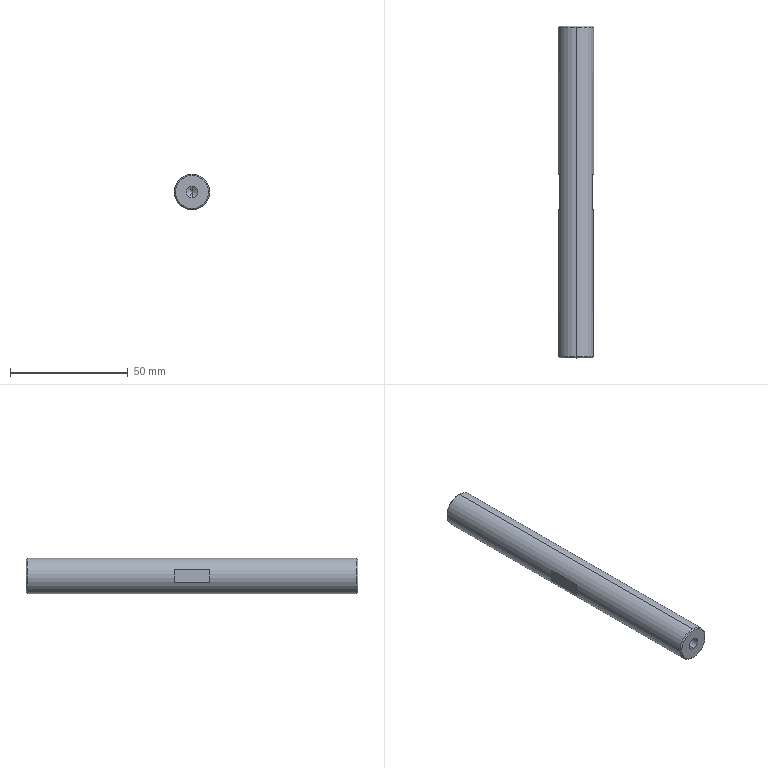Part | STEP file | 0-19-13 Support rod 1 | 1 solid | 22 faces | box 15 x 141 x 15 mm | volume 24242 mm3 | cone 8 | plane 8 | cylinder 6 | commonest cylinder face diameters 5 x4 15 x2
STEP:
#1=CARTESIAN_POINT('',(0.,0.,0.));
#2=DIRECTION('',(0.,0.,1.));
#3=DIRECTION('',(1.,0.,0.));
#4=AXIS2_PLACEMENT_3D('',#1,#2,#3);
#5=CARTESIAN_POINT('',(0.,70.5,7.));
#6=VERTEX_POINT('',#5);
#7=CARTESIAN_POINT('',(0.,70.5,-7.));
#8=VERTEX_POINT('',#7);
#9=CARTESIAN_POINT('',(0.,70.5,0.));
#10=DIRECTION('',(0.,1.,0.));
#11=DIRECTION('',(0.,0.,1.));
#12=AXIS2_PLACEMENT_3D('',#9,#10,#11);
#13=CIRCLE('',#12,7.);
#14=CARTESIAN_POINT('',(0.,70.,0.));
#15=DIRECTION('',(0.,-1.,0.));
#16=DIRECTION('',(0.,0.,-1.));
#17=AXIS2_PLACEMENT_3D('',#14,#15,#16);
#18=CONICAL_SURFACE('',#17,7.5,0.7854);
#19=CARTESIAN_POINT('',(3.142,-0.5));
#20=DIRECTION('',(-1.,0.));
#21=VECTOR('',#20,1.);
#22=LINE('',#19,#21);
#23=(GEOMETRIC_REPRESENTATION_CONTEXT(2)PARAMETRIC_REPRESENTATION_CONTEXT()REPRESENTATION_CONTEXT('',''));
#24=DEFINITIONAL_REPRESENTATION('',(#22),#23);
#25=PCURVE('',#18,#24);
#26=CARTESIAN_POINT('',(7.5,70.5,0.));
#27=DIRECTION('',(0.,1.,0.));
#28=DIRECTION('',(0.,0.,1.));
#29=AXIS2_PLACEMENT_3D('',#26,#27,#28);
#30=PLANE('',#29);
#31=CARTESIAN_POINT('',(0.,-7.5));
#32=DIRECTION('',(1.,0.));
#33=AXIS2_PLACEMENT_2D('',#31,#32);
#34=CIRCLE('',#33,7.);
#35=(GEOMETRIC_REPRESENTATION_CONTEXT(2)PARAMETRIC_REPRESENTATION_CONTEXT()REPRESENTATION_CONTEXT('',''));
#36=DEFINITIONAL_REPRESENTATION('',(#34),#35);
#37=PCURVE('',#30,#36);
#38=SURFACE_CURVE('',#13,(#25,#37),.PCURVE_S1.);
#39=EDGE_CURVE('',#6,#8,#38,.T.);
#40=ORIENTED_EDGE('',*,*,#39,.F.);
#41=CARTESIAN_POINT('',(0.,70.,7.5));
#42=VERTEX_POINT('',#41);
#43=CARTESIAN_POINT('',(0.,70.,7.5));
#44=DIRECTION('',(0.,-0.7071,0.7071));
#45=VECTOR('',#44,1.);
#46=LINE('',#43,#45);
#47=CARTESIAN_POINT('',(3.142,0.));
#48=DIRECTION('',(0.,1.));
#49=VECTOR('',#48,1.);
#50=LINE('',#47,#49);
#51=(GEOMETRIC_REPRESENTATION_CONTEXT(2)PARAMETRIC_REPRESENTATION_CONTEXT()REPRESENTATION_CONTEXT('',''));
#52=DEFINITIONAL_REPRESENTATION('',(#50),#51);
#53=PCURVE('',#18,#52);
#54=CARTESIAN_POINT('',(0.,70.,0.));
#55=DIRECTION('',(0.,-1.,0.));
#56=DIRECTION('',(0.,0.,-1.));
#57=AXIS2_PLACEMENT_3D('',#54,#55,#56);
#58=CONICAL_SURFACE('',#57,7.5,0.7854);
#59=CARTESIAN_POINT('',(3.142,0.));
#60=DIRECTION('',(0.,1.));
#61=VECTOR('',#60,1.);
#62=LINE('',#59,#61);
#63=(GEOMETRIC_REPRESENTATION_CONTEXT(2)PARAMETRIC_REPRESENTATION_CONTEXT()REPRESENTATION_CONTEXT('',''));
#64=DEFINITIONAL_REPRESENTATION('',(#62),#63);
#65=PCURVE('',#58,#64);
#66=SURFACE_CURVE('',#46,(#53,#65),.PCURVE_S1.);
#67=EDGE_CURVE('',#6,#42,#66,.T.);
#68=ORIENTED_EDGE('',*,*,#67,.T.);
#69=CARTESIAN_POINT('',(0.,70.,-7.5));
#70=VERTEX_POINT('',#69);
#71=CARTESIAN_POINT('',(0.,70.,0.));
#72=DIRECTION('',(0.,-1.,0.));
#73=DIRECTION('',(0.,0.,1.));
#74=AXIS2_PLACEMENT_3D('',#71,#72,#73);
#75=CIRCLE('',#74,7.5);
#76=CARTESIAN_POINT('',(-3.142,0.));
#77=DIRECTION('',(1.,0.));
#78=VECTOR('',#77,1.);
#79=LINE('',#76,#78);
#80=(GEOMETRIC_REPRESENTATION_CONTEXT(2)PARAMETRIC_REPRESENTATION_CONTEXT()REPRESENTATION_CONTEXT('',''));
#81=DEFINITIONAL_REPRESENTATION('',(#79),#80);
#82=PCURVE('',#18,#81);
#83=CARTESIAN_POINT('',(0.,0.,0.));
#84=DIRECTION('',(0.,-1.,0.));
#85=DIRECTION('',(0.,0.,-1.));
#86=AXIS2_PLACEMENT_3D('',#83,#84,#85);
#87=CYLINDRICAL_SURFACE('',#86,7.5);
#88=CARTESIAN_POINT('',(-3.142,-70.));
#89=DIRECTION('',(1.,0.));
#90=VECTOR('',#89,1.);
#91=LINE('',#88,#90);
#92=(GEOMETRIC_REPRESENTATION_CONTEXT(2)PARAMETRIC_REPRESENTATION_CONTEXT()REPRESENTATION_CONTEXT('',''));
#93=DEFINITIONAL_REPRESENTATION('',(#91),#92);
#94=PCURVE('',#87,#93);
#95=SURFACE_CURVE('',#75,(#82,#94),.PCURVE_S1.);
#96=EDGE_CURVE('',#70,#42,#95,.T.);
#97=ORIENTED_EDGE('',*,*,#96,.F.);
#98=CARTESIAN_POINT('',(0.,70.,-7.5));
#99=DIRECTION('',(0.,-0.7071,-0.7071));
#100=VECTOR('',#99,1.);
#101=LINE('',#98,#100);
#102=CARTESIAN_POINT('',(0.,0.));
#103=DIRECTION('',(0.,1.));
#104=VECTOR('',#103,1.);
#105=LINE('',#102,#104);
#106=(GEOMETRIC_REPRESENTATION_CONTEXT(2)PARAMETRIC_REPRESENTATION_CONTEXT()REPRESENTATION_CONTEXT('',''));
#107=DEFINITIONAL_REPRESENTATION('',(#105),#106);
#108=PCURVE('',#18,#107);
#109=CARTESIAN_POINT('',(6.283,0.));
#110=DIRECTION('',(0.,1.));
#111=VECTOR('',#110,1.);
#112=LINE('',#109,#111);
#113=(GEOMETRIC_REPRESENTATION_CONTEXT(2)PARAMETRIC_REPRESENTATION_CONTEXT()REPRESENTATION_CONTEXT('',''));
#114=DEFINITIONAL_REPRESENTATION('',(#112),#113);
#115=PCURVE('',#58,#114);
#116=SURFACE_CURVE('',#101,(#108,#115),.PCURVE_S1.);
#117=EDGE_CURVE('',#8,#70,#116,.T.);
#118=ORIENTED_EDGE('',*,*,#117,.F.);
#119=EDGE_LOOP('',(#40,#68,#97,#118));
#120=FACE_BOUND('',#119,.T.);
#121=ADVANCED_FACE('',(#120),#18,.T.);
#122=CARTESIAN_POINT('',(0.,-70.5,-7.));
#123=VERTEX_POINT('',#122);
#124=CARTESIAN_POINT('',(0.,-70.5,7.));
#125=VERTEX_POINT('',#124);
#126=CARTESIAN_POINT('',(0.,-70.5,0.));
#127=DIRECTION('',(0.,-1.,0.));
#128=DIRECTION('',(0.,0.,-1.));
#129=AXIS2_PLACEMENT_3D('',#126,#127,#128);
#130=CIRCLE('',#129,7.);
#131=CARTESIAN_POINT('',(0.,-70.5,0.));
#132=DIRECTION('',(0.,1.,0.));
#133=DIRECTION('',(0.,0.,1.));
#134=AXIS2_PLACEMENT_3D('',#131,#132,#133);
#135=CONICAL_SURFACE('',#134,7.,0.7854);
#136=CARTESIAN_POINT('',(3.142,0.));
#137=DIRECTION('',(-1.,0.));
#138=VECTOR('',#137,1.);
#139=LINE('',#136,#138);
#140=(GEOMETRIC_REPRESENTATION_CONTEXT(2)PARAMETRIC_REPRESENTATION_CONTEXT()REPRESENTATION_CONTEXT('',''));
#141=DEFINITIONAL_REPRESENTATION('',(#139),#140);
#142=PCURVE('',#135,#141);
#143=CARTESIAN_POINT('',(7.5,-70.5,0.));
#144=DIRECTION('',(0.,-1.,0.));
#145=DIRECTION('',(0.,0.,-1.));
#146=AXIS2_PLACEMENT_3D('',#143,#144,#145);
#147=PLANE('',#146);
#148=CARTESIAN_POINT('',(0.,-7.5));
#149=DIRECTION('',(1.,0.));
#150=AXIS2_PLACEMENT_2D('',#148,#149);
#151=CIRCLE('',#150,7.);
#152=(GEOMETRIC_REPRESENTATION_CONTEXT(2)PARAMETRIC_REPRESENTATION_CONTEXT()REPRESENTATION_CONTEXT('',''));
#153=DEFINITIONAL_REPRESENTATION('',(#151),#152);
#154=PCURVE('',#147,#153);
#155=SURFACE_CURVE('',#130,(#142,#154),.PCURVE_S1.);
#156=EDGE_CURVE('',#123,#125,#155,.T.);
#157=ORIENTED_EDGE('',*,*,#156,.F.);
#158=CARTESIAN_POINT('',(0.,-70.,-7.5));
#159=VERTEX_POINT('',#158);
#160=CARTESIAN_POINT('',(0.,-70.5,-7.));
#161=DIRECTION('',(0.,0.7071,-0.7071));
#162=VECTOR('',#161,1.);
#163=LINE('',#160,#162);
#164=CARTESIAN_POINT('',(3.142,0.));
#165=DIRECTION('',(0.,1.));
#166=VECTOR('',#165,1.);
#167=LINE('',#164,#166);
#168=(GEOMETRIC_REPRESENTATION_CONTEXT(2)PARAMETRIC_REPRESENTATION_CONTEXT()REPRESENTATION_CONTEXT('',''));
#169=DEFINITIONAL_REPRESENTATION('',(#167),#168);
#170=PCURVE('',#135,#169);
#171=CARTESIAN_POINT('',(0.,-70.5,0.));
#172=DIRECTION('',(0.,1.,0.));
#173=DIRECTION('',(0.,0.,1.));
#174=AXIS2_PLACEMENT_3D('',#171,#172,#173);
#175=CONICAL_SURFACE('',#174,7.,0.7854);
#176=CARTESIAN_POINT('',(3.142,0.));
#177=DIRECTION('',(0.,1.));
#178=VECTOR('',#177,1.);
#179=LINE('',#176,#178);
#180=(GEOMETRIC_REPRESENTATION_CONTEXT(2)PARAMETRIC_REPRESENTATION_CONTEXT()REPRESENTATION_CONTEXT('',''));
#181=DEFINITIONAL_REPRESENTATION('',(#179),#180);
#182=PCURVE('',#175,#181);
#183=SURFACE_CURVE('',#163,(#170,#182),.PCURVE_S1.);
#184=EDGE_CURVE('',#123,#159,#183,.T.);
#185=ORIENTED_EDGE('',*,*,#184,.T.);
#186=CARTESIAN_POINT('',(0.,-70.,7.5));
#187=VERTEX_POINT('',#186);
#188=CARTESIAN_POINT('',(0.,-70.,0.));
#189=DIRECTION('',(0.,1.,0.));
#190=DIRECTION('',(0.,0.,-1.));
#191=AXIS2_PLACEMENT_3D('',#188,#189,#190);
#192=CIRCLE('',#191,7.5);
#193=CARTESIAN_POINT('',(-3.142,0.5));
#194=DIRECTION('',(1.,0.));
#195=VECTOR('',#194,1.);
#196=LINE('',#193,#195);
#197=(GEOMETRIC_REPRESENTATION_CONTEXT(2)PARAMETRIC_REPRESENTATION_CONTEXT()REPRESENTATION_CONTEXT('',''));
#198=DEFINITIONAL_REPRESENTATION('',(#196),#197);
#199=PCURVE('',#135,#198);
#200=CARTESIAN_POINT('',(6.283,70.));
#201=DIRECTION('',(-1.,0.));
#202=VECTOR('',#201,1.);
#203=LINE('',#200,#202);
#204=(GEOMETRIC_REPRESENTATION_CONTEXT(2)PARAMETRIC_REPRESENTATION_CONTEXT()REPRESENTATION_CONTEXT('',''));
#205=DEFINITIONAL_REPRESENTATION('',(#203),#204);
#206=PCURVE('',#87,#205);
#207=SURFACE_CURVE('',#192,(#199,#206),.PCURVE_S1.);
#208=EDGE_CURVE('',#187,#159,#207,.T.);
#209=ORIENTED_EDGE('',*,*,#208,.F.);
#210=CARTESIAN_POINT('',(0.,-70.5,7.));
#211=DIRECTION('',(0.,0.7071,0.7071));
#212=VECTOR('',#211,1.);
#213=LINE('',#210,#212);
#214=CARTESIAN_POINT('',(0.,0.));
#215=DIRECTION('',(0.,1.));
#216=VECTOR('',#215,1.);
#217=LINE('',#214,#216);
#218=(GEOMETRIC_REPRESENTATION_CONTEXT(2)PARAMETRIC_REPRESENTATION_CONTEXT()REPRESENTATION_CONTEXT('',''));
#219=DEFINITIONAL_REPRESENTATION('',(#217),#218);
#220=PCURVE('',#135,#219);
#221=CARTESIAN_POINT('',(6.283,0.));
#222=DIRECTION('',(0.,1.));
#223=VECTOR('',#222,1.);
#224=LINE('',#221,#223);
#225=(GEOMETRIC_REPRESENTATION_CONTEXT(2)PARAMETRIC_REPRESENTATION_CONTEXT()REPRESENTATION_CONTEXT('',''));
#226=DEFINITIONAL_REPRESENTATION('',(#224),#225);
#227=PCURVE('',#175,#226);
#228=SURFACE_CURVE('',#213,(#220,#227),.PCURVE_S1.);
#229=EDGE_CURVE('',#125,#187,#228,.T.);
#230=ORIENTED_EDGE('',*,*,#229,.F.);
#231=EDGE_LOOP('',(#157,#185,#209,#230));
#232=FACE_BOUND('',#231,.T.);
#233=ADVANCED_FACE('',(#232),#135,.T.);
#234=CARTESIAN_POINT('',(0.,-55.5,-2.5));
#235=VERTEX_POINT('',#234);
#236=CARTESIAN_POINT('',(0.,-70.5,-2.5));
#237=VERTEX_POINT('',#236);
#238=CARTESIAN_POINT('',(0.,-70.5,-2.5));
#239=DIRECTION('',(0.,-1.,0.));
#240=VECTOR('',#239,1.);
#241=LINE('',#238,#240);
#242=CARTESIAN_POINT('',(0.,-70.5,0.));
#243=DIRECTION('',(0.,-1.,0.));
#244=DIRECTION('',(0.,0.,-1.));
#245=AXIS2_PLACEMENT_3D('',#242,#243,#244);
#246=CYLINDRICAL_SURFACE('',#245,2.5);
#247=CARTESIAN_POINT('',(6.283,0.));
#248=DIRECTION('',(0.,1.));
#249=VECTOR('',#248,1.);
#250=LINE('',#247,#249);
#251=(GEOMETRIC_REPRESENTATION_CONTEXT(2)PARAMETRIC_REPRESENTATION_CONTEXT()REPRESENTATION_CONTEXT('',''));
#252=DEFINITIONAL_REPRESENTATION('',(#250),#251);
#253=PCURVE('',#246,#252);
#254=CARTESIAN_POINT('',(0.,-70.5,0.));
#255=DIRECTION('',(0.,-1.,0.));
#256=DIRECTION('',(0.,0.,-1.));
#257=AXIS2_PLACEMENT_3D('',#254,#255,#256);
#258=CYLINDRICAL_SURFACE('',#257,2.5);
#259=CARTESIAN_POINT('',(0.,0.));
#260=DIRECTION('',(0.,1.));
#261=VECTOR('',#260,1.);
#262=LINE('',#259,#261);
#263=(GEOMETRIC_REPRESENTATION_CONTEXT(2)PARAMETRIC_REPRESENTATION_CONTEXT()REPRESENTATION_CONTEXT('',''));
#264=DEFINITIONAL_REPRESENTATION('',(#262),#263);
#265=PCURVE('',#258,#264);
#266=SURFACE_CURVE('',#241,(#253,#265),.PCURVE_S1.);
#267=EDGE_CURVE('',#235,#237,#266,.T.);
#268=ORIENTED_EDGE('',*,*,#267,.T.);
#269=CARTESIAN_POINT('',(0.,-70.5,2.5));
#270=VERTEX_POINT('',#269);
#271=CARTESIAN_POINT('',(0.,-70.5,0.));
#272=DIRECTION('',(0.,-1.,0.));
#273=DIRECTION('',(0.,0.,-1.));
#274=AXIS2_PLACEMENT_3D('',#271,#272,#273);
#275=CIRCLE('',#274,2.5);
#276=CARTESIAN_POINT('',(0.,0.));
#277=DIRECTION('',(1.,0.));
#278=VECTOR('',#277,1.);
#279=LINE('',#276,#278);
#280=(GEOMETRIC_REPRESENTATION_CONTEXT(2)PARAMETRIC_REPRESENTATION_CONTEXT()REPRESENTATION_CONTEXT('',''));
#281=DEFINITIONAL_REPRESENTATION('',(#279),#280);
#282=PCURVE('',#246,#281);
#283=CARTESIAN_POINT('',(0.,-7.5));
#284=DIRECTION('',(1.,0.));
#285=AXIS2_PLACEMENT_2D('',#283,#284);
#286=CIRCLE('',#285,2.5);
#287=(GEOMETRIC_REPRESENTATION_CONTEXT(2)PARAMETRIC_REPRESENTATION_CONTEXT()REPRESENTATION_CONTEXT('',''));
#288=DEFINITIONAL_REPRESENTATION('',(#286),#287);
#289=PCURVE('',#147,#288);
#290=SURFACE_CURVE('',#275,(#282,#289),.PCURVE_S1.);
#291=EDGE_CURVE('',#270,#237,#290,.T.);
#292=ORIENTED_EDGE('',*,*,#291,.F.);
#293=CARTESIAN_POINT('',(0.,-55.5,2.5));
#294=VERTEX_POINT('',#293);
#295=CARTESIAN_POINT('',(0.,-70.5,2.5));
#296=DIRECTION('',(0.,-1.,0.));
#297=VECTOR('',#296,1.);
#298=LINE('',#295,#297);
#299=CARTESIAN_POINT('',(3.142,0.));
#300=DIRECTION('',(0.,1.));
#301=VECTOR('',#300,1.);
#302=LINE('',#299,#301);
#303=(GEOMETRIC_REPRESENTATION_CONTEXT(2)PARAMETRIC_REPRESENTATION_CONTEXT()REPRESENTATION_CONTEXT('',''));
#304=DEFINITIONAL_REPRESENTATION('',(#302),#303);
#305=PCURVE('',#246,#304);
#306=CARTESIAN_POINT('',(3.142,0.));
#307=DIRECTION('',(0.,1.));
#308=VECTOR('',#307,1.);
#309=LINE('',#306,#308);
#310=(GEOMETRIC_REPRESENTATION_CONTEXT(2)PARAMETRIC_REPRESENTATION_CONTEXT()REPRESENTATION_CONTEXT('',''));
#311=DEFINITIONAL_REPRESENTATION('',(#309),#310);
#312=PCURVE('',#258,#311);
#313=SURFACE_CURVE('',#298,(#305,#312),.PCURVE_S1.);
#314=EDGE_CURVE('',#294,#270,#313,.T.);
#315=ORIENTED_EDGE('',*,*,#314,.F.);
#316=CARTESIAN_POINT('',(0.,-55.5,0.));
#317=DIRECTION('',(0.,-1.,0.));
#318=DIRECTION('',(0.,0.,-1.));
#319=AXIS2_PLACEMENT_3D('',#316,#317,#318);
#320=CIRCLE('',#319,2.5);
#321=CARTESIAN_POINT('',(0.,-15.));
#322=DIRECTION('',(1.,0.));
#323=VECTOR('',#322,1.);
#324=LINE('',#321,#323);
#325=(GEOMETRIC_REPRESENTATION_CONTEXT(2)PARAMETRIC_REPRESENTATION_CONTEXT()REPRESENTATION_CONTEXT('',''));
#326=DEFINITIONAL_REPRESENTATION('',(#324),#325);
#327=PCURVE('',#246,#326);
#328=CARTESIAN_POINT('',(0.,-55.5,0.));
#329=DIRECTION('',(0.,-1.,0.));
#330=DIRECTION('',(0.,0.,-1.));
#331=AXIS2_PLACEMENT_3D('',#328,#329,#330);
#332=CONICAL_SURFACE('',#331,2.5,1.03);
#333=CARTESIAN_POINT('',(0.,0.));
#334=DIRECTION('',(1.,0.));
#335=VECTOR('',#334,1.);
#336=LINE('',#333,#335);
#337=(GEOMETRIC_REPRESENTATION_CONTEXT(2)PARAMETRIC_REPRESENTATION_CONTEXT()REPRESENTATION_CONTEXT('',''));
#338=DEFINITIONAL_REPRESENTATION('',(#336),#337);
#339=PCURVE('',#332,#338);
#340=SURFACE_CURVE('',#320,(#327,#339),.PCURVE_S1.);
#341=EDGE_CURVE('',#294,#235,#340,.T.);
#342=ORIENTED_EDGE('',*,*,#341,.T.);
#343=EDGE_LOOP('',(#268,#292,#315,#342));
#344=FACE_BOUND('',#343,.F.);
#345=ADVANCED_FACE('',(#344),#246,.F.);
#346=ORIENTED_EDGE('',*,*,#341,.F.);
#347=CARTESIAN_POINT('',(0.,-53.998,0.));
#348=VERTEX_POINT('',#347);
#349=CARTESIAN_POINT('',(0.,-55.5,2.5));
#350=DIRECTION('',(0.,-0.515,0.8572));
#351=VECTOR('',#350,1.);
#352=LINE('',#349,#351);
#353=CARTESIAN_POINT('',(3.142,0.));
#354=DIRECTION('',(0.,1.));
#355=VECTOR('',#354,1.);
#356=LINE('',#353,#355);
#357=(GEOMETRIC_REPRESENTATION_CONTEXT(2)PARAMETRIC_REPRESENTATION_CONTEXT()REPRESENTATION_CONTEXT('',''));
#358=DEFINITIONAL_REPRESENTATION('',(#356),#357);
#359=PCURVE('',#332,#358);
#360=CARTESIAN_POINT('',(0.,-55.5,0.));
#361=DIRECTION('',(0.,-1.,0.));
#362=DIRECTION('',(0.,0.,-1.));
#363=AXIS2_PLACEMENT_3D('',#360,#361,#362);
#364=CONICAL_SURFACE('',#363,2.5,1.03);
#365=CARTESIAN_POINT('',(3.142,0.));
#366=DIRECTION('',(0.,1.));
#367=VECTOR('',#366,1.);
#368=LINE('',#365,#367);
#369=(GEOMETRIC_REPRESENTATION_CONTEXT(2)PARAMETRIC_REPRESENTATION_CONTEXT()REPRESENTATION_CONTEXT('',''));
#370=DEFINITIONAL_REPRESENTATION('',(#368),#369);
#371=PCURVE('',#364,#370);
#372=SURFACE_CURVE('',#352,(#359,#371),.PCURVE_S1.);
#373=EDGE_CURVE('',#348,#294,#372,.T.);
#374=ORIENTED_EDGE('',*,*,#373,.F.);
#375=CARTESIAN_POINT('',(0.,-55.5,-2.5));
#376=DIRECTION('',(0.,-0.515,-0.8572));
#377=VECTOR('',#376,1.);
#378=LINE('',#375,#377);
#379=CARTESIAN_POINT('',(6.283,0.));
#380=DIRECTION('',(0.,1.));
#381=VECTOR('',#380,1.);
#382=LINE('',#379,#381);
#383=(GEOMETRIC_REPRESENTATION_CONTEXT(2)PARAMETRIC_REPRESENTATION_CONTEXT()REPRESENTATION_CONTEXT('',''));
#384=DEFINITIONAL_REPRESENTATION('',(#382),#383);
#385=PCURVE('',#332,#384);
#386=CARTESIAN_POINT('',(0.,0.));
#387=DIRECTION('',(0.,1.));
#388=VECTOR('',#387,1.);
#389=LINE('',#386,#388);
#390=(GEOMETRIC_REPRESENTATION_CONTEXT(2)PARAMETRIC_REPRESENTATION_CONTEXT()REPRESENTATION_CONTEXT('',''));
#391=DEFINITIONAL_REPRESENTATION('',(#389),#390);
#392=PCURVE('',#364,#391);
#393=SURFACE_CURVE('',#378,(#385,#392),.PCURVE_S1.);
#394=EDGE_CURVE('',#348,#235,#393,.T.);
#395=ORIENTED_EDGE('',*,*,#394,.T.);
#396=EDGE_LOOP('',(#346,#374,#395));
#397=FACE_BOUND('',#396,.F.);
#398=ADVANCED_FACE('',(#397),#332,.F.);
#399=CARTESIAN_POINT('',(0.,55.5,2.5));
#400=VERTEX_POINT('',#399);
#401=CARTESIAN_POINT('',(0.,70.5,2.5));
#402=VERTEX_POINT('',#401);
#403=CARTESIAN_POINT('',(0.,70.5,2.5));
#404=DIRECTION('',(0.,1.,0.));
#405=VECTOR('',#404,1.);
#406=LINE('',#403,#405);
#407=CARTESIAN_POINT('',(0.,70.5,0.));
#408=DIRECTION('',(0.,1.,0.));
#409=DIRECTION('',(0.,0.,1.));
#410=AXIS2_PLACEMENT_3D('',#407,#408,#409);
#411=CYLINDRICAL_SURFACE('',#410,2.5);
#412=CARTESIAN_POINT('',(6.283,0.));
#413=DIRECTION('',(0.,1.));
#414=VECTOR('',#413,1.);
#415=LINE('',#412,#414);
#416=(GEOMETRIC_REPRESENTATION_CONTEXT(2)PARAMETRIC_REPRESENTATION_CONTEXT()REPRESENTATION_CONTEXT('',''));
#417=DEFINITIONAL_REPRESENTATION('',(#415),#416);
#418=PCURVE('',#411,#417);
#419=CARTESIAN_POINT('',(0.,70.5,0.));
#420=DIRECTION('',(0.,1.,0.));
#421=DIRECTION('',(0.,0.,1.));
#422=AXIS2_PLACEMENT_3D('',#419,#420,#421);
#423=CYLINDRICAL_SURFACE('',#422,2.5);
#424=CARTESIAN_POINT('',(0.,0.));
#425=DIRECTION('',(0.,1.));
#426=VECTOR('',#425,1.);
#427=LINE('',#424,#426);
#428=(GEOMETRIC_REPRESENTATION_CONTEXT(2)PARAMETRIC_REPRESENTATION_CONTEXT()REPRESENTATION_CONTEXT('',''));
#429=DEFINITIONAL_REPRESENTATION('',(#427),#428);
#430=PCURVE('',#423,#429);
#431=SURFACE_CURVE('',#406,(#418,#430),.PCURVE_S1.);
#432=EDGE_CURVE('',#400,#402,#431,.T.);
#433=ORIENTED_EDGE('',*,*,#432,.T.);
#434=CARTESIAN_POINT('',(0.,70.5,-2.5));
#435=VERTEX_POINT('',#434);
#436=CARTESIAN_POINT('',(0.,70.5,0.));
#437=DIRECTION('',(0.,1.,0.));
#438=DIRECTION('',(0.,0.,1.));
#439=AXIS2_PLACEMENT_3D('',#436,#437,#438);
#440=CIRCLE('',#439,2.5);
#441=CARTESIAN_POINT('',(0.,0.));
#442=DIRECTION('',(1.,0.));
#443=VECTOR('',#442,1.);
#444=LINE('',#441,#443);
#445=(GEOMETRIC_REPRESENTATION_CONTEXT(2)PARAMETRIC_REPRESENTATION_CONTEXT()REPRESENTATION_CONTEXT('',''));
#446=DEFINITIONAL_REPRESENTATION('',(#444),#445);
#447=PCURVE('',#411,#446);
#448=CARTESIAN_POINT('',(0.,-7.5));
#449=DIRECTION('',(1.,0.));
#450=AXIS2_PLACEMENT_2D('',#448,#449);
#451=CIRCLE('',#450,2.5);
#452=(GEOMETRIC_REPRESENTATION_CONTEXT(2)PARAMETRIC_REPRESENTATION_CONTEXT()REPRESENTATION_CONTEXT('',''));
#453=DEFINITIONAL_REPRESENTATION('',(#451),#452);
#454=PCURVE('',#30,#453);
#455=SURFACE_CURVE('',#440,(#447,#454),.PCURVE_S1.);
#456=EDGE_CURVE('',#435,#402,#455,.T.);
#457=ORIENTED_EDGE('',*,*,#456,.F.);
#458=CARTESIAN_POINT('',(0.,55.5,-2.5));
#459=VERTEX_POINT('',#458);
#460=CARTESIAN_POINT('',(0.,70.5,-2.5));
#461=DIRECTION('',(0.,1.,0.));
#462=VECTOR('',#461,1.);
#463=LINE('',#460,#462);
#464=CARTESIAN_POINT('',(3.142,0.));
#465=DIRECTION('',(0.,1.));
#466=VECTOR('',#465,1.);
#467=LINE('',#464,#466);
#468=(GEOMETRIC_REPRESENTATION_CONTEXT(2)PARAMETRIC_REPRESENTATION_CONTEXT()REPRESENTATION_CONTEXT('',''));
#469=DEFINITIONAL_REPRESENTATION('',(#467),#468);
#470=PCURVE('',#411,#469);
#471=CARTESIAN_POINT('',(3.142,0.));
#472=DIRECTION('',(0.,1.));
#473=VECTOR('',#472,1.);
#474=LINE('',#471,#473);
#475=(GEOMETRIC_REPRESENTATION_CONTEXT(2)PARAMETRIC_REPRESENTATION_CONTEXT()REPRESENTATION_CONTEXT('',''));
#476=DEFINITIONAL_REPRESENTATION('',(#474),#475);
#477=PCURVE('',#423,#476);
#478=SURFACE_CURVE('',#463,(#470,#477),.PCURVE_S1.);
#479=EDGE_CURVE('',#459,#435,#478,.T.);
#480=ORIENTED_EDGE('',*,*,#479,.F.);
#481=CARTESIAN_POINT('',(0.,55.5,0.));
#482=DIRECTION('',(0.,1.,0.));
#483=DIRECTION('',(0.,0.,1.));
#484=AXIS2_PLACEMENT_3D('',#481,#482,#483);
#485=CIRCLE('',#484,2.5);
#486=CARTESIAN_POINT('',(0.,-15.));
#487=DIRECTION('',(1.,0.));
#488=VECTOR('',#487,1.);
#489=LINE('',#486,#488);
#490=(GEOMETRIC_REPRESENTATION_CONTEXT(2)PARAMETRIC_REPRESENTATION_CONTEXT()REPRESENTATION_CONTEXT('',''));
#491=DEFINITIONAL_REPRESENTATION('',(#489),#490);
#492=PCURVE('',#411,#491);
#493=CARTESIAN_POINT('',(0.,55.5,0.));
#494=DIRECTION('',(0.,1.,0.));
#495=DIRECTION('',(0.,0.,1.));
#496=AXIS2_PLACEMENT_3D('',#493,#494,#495);
#497=CONICAL_SURFACE('',#496,2.5,1.03);
#498=CARTESIAN_POINT('',(0.,0.));
#499=DIRECTION('',(1.,0.));
#500=VECTOR('',#499,1.);
#501=LINE('',#498,#500);
#502=(GEOMETRIC_REPRESENTATION_CONTEXT(2)PARAMETRIC_REPRESENTATION_CONTEXT()REPRESENTATION_CONTEXT('',''));
#503=DEFINITIONAL_REPRESENTATION('',(#501),#502);
#504=PCURVE('',#497,#503);
#505=SURFACE_CURVE('',#485,(#492,#504),.PCURVE_S1.);
#506=EDGE_CURVE('',#459,#400,#505,.T.);
#507=ORIENTED_EDGE('',*,*,#506,.T.);
#508=EDGE_LOOP('',(#433,#457,#480,#507));
#509=FACE_BOUND('',#508,.F.);
#510=ADVANCED_FACE('',(#509),#411,.F.);
#511=ORIENTED_EDGE('',*,*,#506,.F.);
#512=CARTESIAN_POINT('',(0.,53.998,0.));
#513=VERTEX_POINT('',#512);
#514=CARTESIAN_POINT('',(0.,55.5,-2.5));
#515=DIRECTION('',(0.,0.515,-0.8572));
#516=VECTOR('',#515,1.);
#517=LINE('',#514,#516);
#518=CARTESIAN_POINT('',(3.142,0.));
#519=DIRECTION('',(0.,1.));
#520=VECTOR('',#519,1.);
#521=LINE('',#518,#520);
#522=(GEOMETRIC_REPRESENTATION_CONTEXT(2)PARAMETRIC_REPRESENTATION_CONTEXT()REPRESENTATION_CONTEXT('',''));
#523=DEFINITIONAL_REPRESENTATION('',(#521),#522);
#524=PCURVE('',#497,#523);
#525=CARTESIAN_POINT('',(0.,55.5,0.));
#526=DIRECTION('',(0.,1.,0.));
#527=DIRECTION('',(0.,0.,1.));
#528=AXIS2_PLACEMENT_3D('',#525,#526,#527);
#529=CONICAL_SURFACE('',#528,2.5,1.03);
#530=CARTESIAN_POINT('',(3.142,0.));
#531=DIRECTION('',(0.,1.));
#532=VECTOR('',#531,1.);
#533=LINE('',#530,#532);
#534=(GEOMETRIC_REPRESENTATION_CONTEXT(2)PARAMETRIC_REPRESENTATION_CONTEXT()REPRESENTATION_CONTEXT('',''));
#535=DEFINITIONAL_REPRESENTATION('',(#533),#534);
#536=PCURVE('',#529,#535);
#537=SURFACE_CURVE('',#517,(#524,#536),.PCURVE_S1.);
#538=EDGE_CURVE('',#513,#459,#537,.T.);
#539=ORIENTED_EDGE('',*,*,#538,.F.);
#540=CARTESIAN_POINT('',(0.,55.5,2.5));
#541=DIRECTION('',(0.,0.515,0.8572));
#542=VECTOR('',#541,1.);
#543=LINE('',#540,#542);
#544=CARTESIAN_POINT('',(6.283,0.));
#545=DIRECTION('',(0.,1.));
#546=VECTOR('',#545,1.);
#547=LINE('',#544,#546);
#548=(GEOMETRIC_REPRESENTATION_CONTEXT(2)PARAMETRIC_REPRESENTATION_CONTEXT()REPRESENTATION_CONTEXT('',''));
#549=DEFINITIONAL_REPRESENTATION('',(#547),#548);
#550=PCURVE('',#497,#549);
#551=CARTESIAN_POINT('',(0.,0.));
#552=DIRECTION('',(0.,1.));
#553=VECTOR('',#552,1.);
#554=LINE('',#551,#553);
#555=(GEOMETRIC_REPRESENTATION_CONTEXT(2)PARAMETRIC_REPRESENTATION_CONTEXT()REPRESENTATION_CONTEXT('',''));
#556=DEFINITIONAL_REPRESENTATION('',(#554),#555);
#557=PCURVE('',#529,#556);
#558=SURFACE_CURVE('',#543,(#550,#557),.PCURVE_S1.);
#559=EDGE_CURVE('',#513,#400,#558,.T.);
#560=ORIENTED_EDGE('',*,*,#559,.T.);
#561=EDGE_LOOP('',(#511,#539,#560));
#562=FACE_BOUND('',#561,.F.);
#563=ADVANCED_FACE('',(#562),#497,.F.);
#564=CARTESIAN_POINT('',(7.,-7.5,2.693));
#565=VERTEX_POINT('',#564);
#566=CARTESIAN_POINT('',(7.,-7.5,-2.693));
#567=VERTEX_POINT('',#566);
#568=CARTESIAN_POINT('',(0.,-7.5,0.));
#569=DIRECTION('',(0.,1.,0.));
#570=DIRECTION('',(0.,0.,-1.));
#571=AXIS2_PLACEMENT_3D('',#568,#569,#570);
#572=CIRCLE('',#571,7.5);
#573=CARTESIAN_POINT('',(6.283,7.5));
#574=DIRECTION('',(-1.,0.));
#575=VECTOR('',#574,1.);
#576=LINE('',#573,#575);
#577=(GEOMETRIC_REPRESENTATION_CONTEXT(2)PARAMETRIC_REPRESENTATION_CONTEXT()REPRESENTATION_CONTEXT('',''));
#578=DEFINITIONAL_REPRESENTATION('',(#576),#577);
#579=PCURVE('',#87,#578);
#580=CARTESIAN_POINT('',(0.,-7.5,0.));
#581=DIRECTION('',(0.,-1.,0.));
#582=DIRECTION('',(0.,0.,-1.));
#583=AXIS2_PLACEMENT_3D('',#580,#581,#582);
#584=PLANE('',#583);
#585=CARTESIAN_POINT('',(7.5,0.));
#586=CARTESIAN_POINT('',(7.5,-12.99));
#587=CARTESIAN_POINT('',(-3.75,-6.495));
#588=CARTESIAN_POINT('',(-15.,0.));
#589=CARTESIAN_POINT('',(-3.75,6.495));
#590=CARTESIAN_POINT('',(7.5,12.99));
#591=CARTESIAN_POINT('',(7.5,0.));
#592=(BOUNDED_CURVE()B_SPLINE_CURVE(2,(#585,#586,#587,#588,#589,#590,#591),.UNSPECIFIED.,.T.,.F.)B_SPLINE_CURVE_WITH_KNOTS((1,2,2,2,2,1),(-2.094,0.,2.094,4.189,6.283,8.378),.UNSPECIFIED.)CURVE()GEOMETRIC_REPRESENTATION_ITEM()RATIONAL_B_SPLINE_CURVE((1.,0.5,1.,0.5,1.,0.5,1.))REPRESENTATION_ITEM(''));
#593=(GEOMETRIC_REPRESENTATION_CONTEXT(2)PARAMETRIC_REPRESENTATION_CONTEXT()REPRESENTATION_CONTEXT('',''));
#594=DEFINITIONAL_REPRESENTATION('',(#592),#593);
#595=PCURVE('',#584,#594);
#596=SURFACE_CURVE('',#572,(#579,#595),.PCURVE_S1.);
#597=EDGE_CURVE('',#565,#567,#596,.T.);
#598=ORIENTED_EDGE('',*,*,#597,.F.);
#599=CARTESIAN_POINT('',(7.,7.5,2.693));
#600=VERTEX_POINT('',#599);
#601=CARTESIAN_POINT('',(7.,-7.5,2.693));
#602=DIRECTION('',(0.,1.,0.));
#603=VECTOR('',#602,1.);
#604=LINE('',#601,#603);
#605=CARTESIAN_POINT('',(1.938,7.5));
#606=DIRECTION('',(0.,-1.));
#607=VECTOR('',#606,1.);
#608=LINE('',#605,#607);
#609=(GEOMETRIC_REPRESENTATION_CONTEXT(2)PARAMETRIC_REPRESENTATION_CONTEXT()REPRESENTATION_CONTEXT('',''));
#610=DEFINITIONAL_REPRESENTATION('',(#608),#609);
#611=PCURVE('',#87,#610);
#612=CARTESIAN_POINT('',(7.,-7.5,2.693));
#613=DIRECTION('',(-1.,0.,0.));
#614=DIRECTION('',(0.,0.,1.));
#615=AXIS2_PLACEMENT_3D('',#612,#613,#614);
#616=PLANE('',#615);
#617=CARTESIAN_POINT('',(0.,0.));
#618=DIRECTION('',(0.,1.));
#619=VECTOR('',#618,1.);
#620=LINE('',#617,#619);
#621=(GEOMETRIC_REPRESENTATION_CONTEXT(2)PARAMETRIC_REPRESENTATION_CONTEXT()REPRESENTATION_CONTEXT('',''));
#622=DEFINITIONAL_REPRESENTATION('',(#620),#621);
#623=PCURVE('',#616,#622);
#624=SURFACE_CURVE('',#604,(#611,#623),.PCURVE_S1.);
#625=EDGE_CURVE('',#565,#600,#624,.T.);
#626=ORIENTED_EDGE('',*,*,#625,.T.);
#627=CARTESIAN_POINT('',(7.,7.5,-2.693));
#628=VERTEX_POINT('',#627);
#629=CARTESIAN_POINT('',(0.,7.5,0.));
#630=DIRECTION('',(0.,1.,0.));
#631=DIRECTION('',(0.,0.,-1.));
#632=AXIS2_PLACEMENT_3D('',#629,#630,#631);
#633=CIRCLE('',#632,7.5);
#634=CARTESIAN_POINT('',(6.283,-7.5));
#635=DIRECTION('',(-1.,0.));
#636=VECTOR('',#635,1.);
#637=LINE('',#634,#636);
#638=(GEOMETRIC_REPRESENTATION_CONTEXT(2)PARAMETRIC_REPRESENTATION_CONTEXT()REPRESENTATION_CONTEXT('',''));
#639=DEFINITIONAL_REPRESENTATION('',(#637),#638);
#640=PCURVE('',#87,#639);
#641=CARTESIAN_POINT('',(0.,7.5,0.));
#642=DIRECTION('',(0.,-1.,0.));
#643=DIRECTION('',(0.,0.,-1.));
#644=AXIS2_PLACEMENT_3D('',#641,#642,#643);
#645=PLANE('',#644);
#646=CARTESIAN_POINT('',(7.5,0.));
#647=CARTESIAN_POINT('',(7.5,-12.99));
#648=CARTESIAN_POINT('',(-3.75,-6.495));
#649=CARTESIAN_POINT('',(-15.,0.));
#650=CARTESIAN_POINT('',(-3.75,6.495));
#651=CARTESIAN_POINT('',(7.5,12.99));
#652=CARTESIAN_POINT('',(7.5,0.));
#653=(BOUNDED_CURVE()B_SPLINE_CURVE(2,(#646,#647,#648,#649,#650,#651,#652),.UNSPECIFIED.,.T.,.F.)B_SPLINE_CURVE_WITH_KNOTS((1,2,2,2,2,1),(-2.094,0.,2.094,4.189,6.283,8.378),.UNSPECIFIED.)CURVE()GEOMETRIC_REPRESENTATION_ITEM()RATIONAL_B_SPLINE_CURVE((1.,0.5,1.,0.5,1.,0.5,1.))REPRESENTATION_ITEM(''));
#654=(GEOMETRIC_REPRESENTATION_CONTEXT(2)PARAMETRIC_REPRESENTATION_CONTEXT()REPRESENTATION_CONTEXT('',''));
#655=DEFINITIONAL_REPRESENTATION('',(#653),#654);
#656=PCURVE('',#645,#655);
#657=SURFACE_CURVE('',#633,(#640,#656),.PCURVE_S1.);
#658=EDGE_CURVE('',#600,#628,#657,.T.);
#659=ORIENTED_EDGE('',*,*,#658,.T.);
#660=CARTESIAN_POINT('',(7.,-7.5,-2.693));
#661=DIRECTION('',(0.,1.,0.));
#662=VECTOR('',#661,1.);
#663=LINE('',#660,#662);
#664=CARTESIAN_POINT('',(1.204,7.5));
#665=DIRECTION('',(0.,-1.));
#666=VECTOR('',#665,1.);
#667=LINE('',#664,#666);
#668=(GEOMETRIC_REPRESENTATION_CONTEXT(2)PARAMETRIC_REPRESENTATION_CONTEXT()REPRESENTATION_CONTEXT('',''));
#669=DEFINITIONAL_REPRESENTATION('',(#667),#668);
#670=PCURVE('',#87,#669);
#671=CARTESIAN_POINT('',(-5.385,0.));
#672=DIRECTION('',(0.,1.));
#673=VECTOR('',#672,1.);
#674=LINE('',#671,#673);
#675=(GEOMETRIC_REPRESENTATION_CONTEXT(2)PARAMETRIC_REPRESENTATION_CONTEXT()REPRESENTATION_CONTEXT('',''));
#676=DEFINITIONAL_REPRESENTATION('',(#674),#675);
#677=PCURVE('',#616,#676);
#678=SURFACE_CURVE('',#663,(#670,#677),.PCURVE_S1.);
#679=EDGE_CURVE('',#567,#628,#678,.T.);
#680=ORIENTED_EDGE('',*,*,#679,.F.);
#681=EDGE_LOOP('',(#598,#626,#659,#680));
#682=FACE_BOUND('',#681,.T.);
#683=ORIENTED_EDGE('',*,*,#96,.T.);
#684=CARTESIAN_POINT('',(0.,0.,7.5));
#685=DIRECTION('',(0.,-1.,0.));
#686=VECTOR('',#685,1.);
#687=LINE('',#684,#686);
#688=CARTESIAN_POINT('',(3.142,0.));
#689=DIRECTION('',(0.,1.));
#690=VECTOR('',#689,1.);
#691=LINE('',#688,#690);
#692=(GEOMETRIC_REPRESENTATION_CONTEXT(2)PARAMETRIC_REPRESENTATION_CONTEXT()REPRESENTATION_CONTEXT('',''));
#693=DEFINITIONAL_REPRESENTATION('',(#691),#692);
#694=PCURVE('',#87,#693);
#695=CARTESIAN_POINT('',(0.,0.,0.));
#696=DIRECTION('',(0.,-1.,0.));
#697=DIRECTION('',(0.,0.,-1.));
#698=AXIS2_PLACEMENT_3D('',#695,#696,#697);
#699=CYLINDRICAL_SURFACE('',#698,7.5);
#700=CARTESIAN_POINT('',(3.142,0.));
#701=DIRECTION('',(0.,1.));
#702=VECTOR('',#701,1.);
#703=LINE('',#700,#702);
#704=(GEOMETRIC_REPRESENTATION_CONTEXT(2)PARAMETRIC_REPRESENTATION_CONTEXT()REPRESENTATION_CONTEXT('',''));
#705=DEFINITIONAL_REPRESENTATION('',(#703),#704);
#706=PCURVE('',#699,#705);
#707=SURFACE_CURVE('',#687,(#694,#706),.PCURVE_S1.);
#708=EDGE_CURVE('',#42,#187,#707,.T.);
#709=ORIENTED_EDGE('',*,*,#708,.T.);
#710=ORIENTED_EDGE('',*,*,#208,.T.);
#711=CARTESIAN_POINT('',(0.,0.,-7.5));
#712=DIRECTION('',(0.,-1.,0.));
#713=VECTOR('',#712,1.);
#714=LINE('',#711,#713);
#715=CARTESIAN_POINT('',(0.,0.));
#716=DIRECTION('',(0.,1.));
#717=VECTOR('',#716,1.);
#718=LINE('',#715,#717);
#719=(GEOMETRIC_REPRESENTATION_CONTEXT(2)PARAMETRIC_REPRESENTATION_CONTEXT()REPRESENTATION_CONTEXT('',''));
#720=DEFINITIONAL_REPRESENTATION('',(#718),#719);
#721=PCURVE('',#87,#720);
#722=CARTESIAN_POINT('',(6.283,0.));
#723=DIRECTION('',(0.,1.));
#724=VECTOR('',#723,1.);
#725=LINE('',#722,#724);
#726=(GEOMETRIC_REPRESENTATION_CONTEXT(2)PARAMETRIC_REPRESENTATION_CONTEXT()REPRESENTATION_CONTEXT('',''));
#727=DEFINITIONAL_REPRESENTATION('',(#725),#726);
#728=PCURVE('',#699,#727);
#729=SURFACE_CURVE('',#714,(#721,#728),.PCURVE_S1.);
#730=EDGE_CURVE('',#70,#159,#729,.T.);
#731=ORIENTED_EDGE('',*,*,#730,.F.);
#732=EDGE_LOOP('',(#683,#709,#710,#731));
#733=FACE_BOUND('',#732,.T.);
#734=ADVANCED_FACE('',(#682,#733),#87,.T.);
#735=ORIENTED_EDGE('',*,*,#708,.F.);
#736=CARTESIAN_POINT('',(0.,70.,0.));
#737=DIRECTION('',(0.,-1.,0.));
#738=DIRECTION('',(0.,0.,1.));
#739=AXIS2_PLACEMENT_3D('',#736,#737,#738);
#740=CIRCLE('',#739,7.5);
#741=CARTESIAN_POINT('',(3.142,-70.));
#742=DIRECTION('',(1.,0.));
#743=VECTOR('',#742,1.);
#744=LINE('',#741,#743);
#745=(GEOMETRIC_REPRESENTATION_CONTEXT(2)PARAMETRIC_REPRESENTATION_CONTEXT()REPRESENTATION_CONTEXT('',''));
#746=DEFINITIONAL_REPRESENTATION('',(#744),#745);
#747=PCURVE('',#699,#746);
#748=CARTESIAN_POINT('',(3.142,0.));
#749=DIRECTION('',(1.,0.));
#750=VECTOR('',#749,1.);
#751=LINE('',#748,#750);
#752=(GEOMETRIC_REPRESENTATION_CONTEXT(2)PARAMETRIC_REPRESENTATION_CONTEXT()REPRESENTATION_CONTEXT('',''));
#753=DEFINITIONAL_REPRESENTATION('',(#751),#752);
#754=PCURVE('',#58,#753);
#755=SURFACE_CURVE('',#740,(#747,#754),.PCURVE_S1.);
#756=EDGE_CURVE('',#42,#70,#755,.T.);
#757=ORIENTED_EDGE('',*,*,#756,.T.);
#758=ORIENTED_EDGE('',*,*,#730,.T.);
#759=CARTESIAN_POINT('',(0.,-70.,0.));
#760=DIRECTION('',(0.,1.,0.));
#761=DIRECTION('',(0.,0.,-1.));
#762=AXIS2_PLACEMENT_3D('',#759,#760,#761);
#763=CIRCLE('',#762,7.5);
#764=CARTESIAN_POINT('',(6.283,70.));
#765=DIRECTION('',(-1.,0.));
#766=VECTOR('',#765,1.);
#767=LINE('',#764,#766);
#768=(GEOMETRIC_REPRESENTATION_CONTEXT(2)PARAMETRIC_REPRESENTATION_CONTEXT()REPRESENTATION_CONTEXT('',''));
#769=DEFINITIONAL_REPRESENTATION('',(#767),#768);
#770=PCURVE('',#699,#769);
#771=CARTESIAN_POINT('',(3.142,0.5));
#772=DIRECTION('',(1.,0.));
#773=VECTOR('',#772,1.);
#774=LINE('',#771,#773);
#775=(GEOMETRIC_REPRESENTATION_CONTEXT(2)PARAMETRIC_REPRESENTATION_CONTEXT()REPRESENTATION_CONTEXT('',''));
#776=DEFINITIONAL_REPRESENTATION('',(#774),#775);
#777=PCURVE('',#175,#776);
#778=SURFACE_CURVE('',#763,(#770,#777),.PCURVE_S1.);
#779=EDGE_CURVE('',#159,#187,#778,.T.);
#780=ORIENTED_EDGE('',*,*,#779,.T.);
#781=EDGE_LOOP('',(#735,#757,#758,#780));
#782=FACE_BOUND('',#781,.T.);
#783=CARTESIAN_POINT('',(-7.,-7.5,2.693));
#784=VERTEX_POINT('',#783);
#785=CARTESIAN_POINT('',(-7.,7.5,2.693));
#786=VERTEX_POINT('',#785);
#787=CARTESIAN_POINT('',(-7.,-7.5,2.693));
#788=DIRECTION('',(0.,1.,0.));
#789=VECTOR('',#788,1.);
#790=LINE('',#787,#789);
#791=CARTESIAN_POINT('',(4.345,7.5));
#792=DIRECTION('',(0.,-1.));
#793=VECTOR('',#792,1.);
#794=LINE('',#791,#793);
#795=(GEOMETRIC_REPRESENTATION_CONTEXT(2)PARAMETRIC_REPRESENTATION_CONTEXT()REPRESENTATION_CONTEXT('',''));
#796=DEFINITIONAL_REPRESENTATION('',(#794),#795);
#797=PCURVE('',#699,#796);
#798=CARTESIAN_POINT('',(-7.,-7.5,2.693));
#799=DIRECTION('',(1.,0.,0.));
#800=DIRECTION('',(0.,0.,-1.));
#801=AXIS2_PLACEMENT_3D('',#798,#799,#800);
#802=PLANE('',#801);
#803=CARTESIAN_POINT('',(0.,0.));
#804=DIRECTION('',(0.,1.));
#805=VECTOR('',#804,1.);
#806=LINE('',#803,#805);
#807=(GEOMETRIC_REPRESENTATION_CONTEXT(2)PARAMETRIC_REPRESENTATION_CONTEXT()REPRESENTATION_CONTEXT('',''));
#808=DEFINITIONAL_REPRESENTATION('',(#806),#807);
#809=PCURVE('',#802,#808);
#810=SURFACE_CURVE('',#790,(#797,#809),.PCURVE_S1.);
#811=EDGE_CURVE('',#784,#786,#810,.T.);
#812=ORIENTED_EDGE('',*,*,#811,.F.);
#813=CARTESIAN_POINT('',(-7.,-7.5,-2.693));
#814=VERTEX_POINT('',#813);
#815=CARTESIAN_POINT('',(0.,-7.5,0.));
#816=DIRECTION('',(0.,-1.,0.));
#817=DIRECTION('',(0.,0.,1.));
#818=AXIS2_PLACEMENT_3D('',#815,#816,#817);
#819=CIRCLE('',#818,7.5);
#820=CARTESIAN_POINT('',(3.142,7.5));
#821=DIRECTION('',(1.,0.));
#822=VECTOR('',#821,1.);
#823=LINE('',#820,#822);
#824=(GEOMETRIC_REPRESENTATION_CONTEXT(2)PARAMETRIC_REPRESENTATION_CONTEXT()REPRESENTATION_CONTEXT('',''));
#825=DEFINITIONAL_REPRESENTATION('',(#823),#824);
#826=PCURVE('',#699,#825);
#827=CARTESIAN_POINT('',(0.,-7.5,0.));
#828=DIRECTION('',(0.,1.,0.));
#829=DIRECTION('',(0.,0.,1.));
#830=AXIS2_PLACEMENT_3D('',#827,#828,#829);
#831=PLANE('',#830);
#832=CARTESIAN_POINT('',(7.5,0.));
#833=CARTESIAN_POINT('',(7.5,-12.99));
#834=CARTESIAN_POINT('',(-3.75,-6.495));
#835=CARTESIAN_POINT('',(-15.,0.));
#836=CARTESIAN_POINT('',(-3.75,6.495));
#837=CARTESIAN_POINT('',(7.5,12.99));
#838=CARTESIAN_POINT('',(7.5,0.));
#839=(BOUNDED_CURVE()B_SPLINE_CURVE(2,(#832,#833,#834,#835,#836,#837,#838),.UNSPECIFIED.,.T.,.F.)B_SPLINE_CURVE_WITH_KNOTS((1,2,2,2,2,1),(-2.094,0.,2.094,4.189,6.283,8.378),.UNSPECIFIED.)CURVE()GEOMETRIC_REPRESENTATION_ITEM()RATIONAL_B_SPLINE_CURVE((1.,0.5,1.,0.5,1.,0.5,1.))REPRESENTATION_ITEM(''));
#840=(GEOMETRIC_REPRESENTATION_CONTEXT(2)PARAMETRIC_REPRESENTATION_CONTEXT()REPRESENTATION_CONTEXT('',''));
#841=DEFINITIONAL_REPRESENTATION('',(#839),#840);
#842=PCURVE('',#831,#841);
#843=SURFACE_CURVE('',#819,(#826,#842),.PCURVE_S1.);
#844=EDGE_CURVE('',#784,#814,#843,.T.);
#845=ORIENTED_EDGE('',*,*,#844,.T.);
#846=CARTESIAN_POINT('',(-7.,7.5,-2.693));
#847=VERTEX_POINT('',#846);
#848=CARTESIAN_POINT('',(-7.,-7.5,-2.693));
#849=DIRECTION('',(0.,1.,0.));
#850=VECTOR('',#849,1.);
#851=LINE('',#848,#850);
#852=CARTESIAN_POINT('',(5.08,7.5));
#853=DIRECTION('',(0.,-1.));
#854=VECTOR('',#853,1.);
#855=LINE('',#852,#854);
#856=(GEOMETRIC_REPRESENTATION_CONTEXT(2)PARAMETRIC_REPRESENTATION_CONTEXT()REPRESENTATION_CONTEXT('',''));
#857=DEFINITIONAL_REPRESENTATION('',(#855),#856);
#858=PCURVE('',#699,#857);
#859=CARTESIAN_POINT('',(5.385,0.));
#860=DIRECTION('',(0.,1.));
#861=VECTOR('',#860,1.);
#862=LINE('',#859,#861);
#863=(GEOMETRIC_REPRESENTATION_CONTEXT(2)PARAMETRIC_REPRESENTATION_CONTEXT()REPRESENTATION_CONTEXT('',''));
#864=DEFINITIONAL_REPRESENTATION('',(#862),#863);
#865=PCURVE('',#802,#864);
#866=SURFACE_CURVE('',#851,(#858,#865),.PCURVE_S1.);
#867=EDGE_CURVE('',#814,#847,#866,.T.);
#868=ORIENTED_EDGE('',*,*,#867,.T.);
#869=CARTESIAN_POINT('',(0.,7.5,0.));
#870=DIRECTION('',(0.,-1.,0.));
#871=DIRECTION('',(0.,0.,1.));
#872=AXIS2_PLACEMENT_3D('',#869,#870,#871);
#873=CIRCLE('',#872,7.5);
#874=CARTESIAN_POINT('',(3.142,-7.5));
#875=DIRECTION('',(1.,0.));
#876=VECTOR('',#875,1.);
#877=LINE('',#874,#876);
#878=(GEOMETRIC_REPRESENTATION_CONTEXT(2)PARAMETRIC_REPRESENTATION_CONTEXT()REPRESENTATION_CONTEXT('',''));
#879=DEFINITIONAL_REPRESENTATION('',(#877),#878);
#880=PCURVE('',#699,#879);
#881=CARTESIAN_POINT('',(0.,7.5,0.));
#882=DIRECTION('',(0.,1.,0.));
#883=DIRECTION('',(0.,0.,1.));
#884=AXIS2_PLACEMENT_3D('',#881,#882,#883);
#885=PLANE('',#884);
#886=CARTESIAN_POINT('',(7.5,0.));
#887=CARTESIAN_POINT('',(7.5,-12.99));
#888=CARTESIAN_POINT('',(-3.75,-6.495));
#889=CARTESIAN_POINT('',(-15.,0.));
#890=CARTESIAN_POINT('',(-3.75,6.495));
#891=CARTESIAN_POINT('',(7.5,12.99));
#892=CARTESIAN_POINT('',(7.5,0.));
#893=(BOUNDED_CURVE()B_SPLINE_CURVE(2,(#886,#887,#888,#889,#890,#891,#892),.UNSPECIFIED.,.T.,.F.)B_SPLINE_CURVE_WITH_KNOTS((1,2,2,2,2,1),(-2.094,0.,2.094,4.189,6.283,8.378),.UNSPECIFIED.)CURVE()GEOMETRIC_REPRESENTATION_ITEM()RATIONAL_B_SPLINE_CURVE((1.,0.5,1.,0.5,1.,0.5,1.))REPRESENTATION_ITEM(''));
#894=(GEOMETRIC_REPRESENTATION_CONTEXT(2)PARAMETRIC_REPRESENTATION_CONTEXT()REPRESENTATION_CONTEXT('',''));
#895=DEFINITIONAL_REPRESENTATION('',(#893),#894);
#896=PCURVE('',#885,#895);
#897=SURFACE_CURVE('',#873,(#880,#896),.PCURVE_S1.);
#898=EDGE_CURVE('',#786,#847,#897,.T.);
#899=ORIENTED_EDGE('',*,*,#898,.F.);
#900=EDGE_LOOP('',(#812,#845,#868,#899));
#901=FACE_BOUND('',#900,.T.);
#902=ADVANCED_FACE('',(#782,#901),#699,.T.);
#903=CARTESIAN_POINT('',(0.,70.5,0.));
#904=DIRECTION('',(0.,1.,0.));
#905=DIRECTION('',(0.,0.,1.));
#906=AXIS2_PLACEMENT_3D('',#903,#904,#905);
#907=CIRCLE('',#906,7.);
#908=CARTESIAN_POINT('',(0.,-7.5));
#909=DIRECTION('',(1.,0.));
#910=AXIS2_PLACEMENT_2D('',#908,#909);
#911=CIRCLE('',#910,7.);
#912=(GEOMETRIC_REPRESENTATION_CONTEXT(2)PARAMETRIC_REPRESENTATION_CONTEXT()REPRESENTATION_CONTEXT('',''));
#913=DEFINITIONAL_REPRESENTATION('',(#911),#912);
#914=PCURVE('',#30,#913);
#915=CARTESIAN_POINT('',(9.425,-0.5));
#916=DIRECTION('',(-1.,0.));
#917=VECTOR('',#916,1.);
#918=LINE('',#915,#917);
#919=(GEOMETRIC_REPRESENTATION_CONTEXT(2)PARAMETRIC_REPRESENTATION_CONTEXT()REPRESENTATION_CONTEXT('',''));
#920=DEFINITIONAL_REPRESENTATION('',(#918),#919);
#921=PCURVE('',#58,#920);
#922=SURFACE_CURVE('',#907,(#914,#921),.PCURVE_S1.);
#923=EDGE_CURVE('',#8,#6,#922,.T.);
#924=ORIENTED_EDGE('',*,*,#923,.T.);
#925=ORIENTED_EDGE('',*,*,#39,.T.);
#926=EDGE_LOOP('',(#924,#925));
#927=FACE_BOUND('',#926,.T.);
#928=CARTESIAN_POINT('',(0.,70.5,0.));
#929=DIRECTION('',(0.,1.,0.));
#930=DIRECTION('',(0.,0.,1.));
#931=AXIS2_PLACEMENT_3D('',#928,#929,#930);
#932=CIRCLE('',#931,2.5);
#933=CARTESIAN_POINT('',(0.,-7.5));
#934=DIRECTION('',(1.,0.));
#935=AXIS2_PLACEMENT_2D('',#933,#934);
#936=CIRCLE('',#935,2.5);
#937=(GEOMETRIC_REPRESENTATION_CONTEXT(2)PARAMETRIC_REPRESENTATION_CONTEXT()REPRESENTATION_CONTEXT('',''));
#938=DEFINITIONAL_REPRESENTATION('',(#936),#937);
#939=PCURVE('',#30,#938);
#940=CARTESIAN_POINT('',(0.,0.));
#941=DIRECTION('',(1.,0.));
#942=VECTOR('',#941,1.);
#943=LINE('',#940,#942);
#944=(GEOMETRIC_REPRESENTATION_CONTEXT(2)PARAMETRIC_REPRESENTATION_CONTEXT()REPRESENTATION_CONTEXT('',''));
#945=DEFINITIONAL_REPRESENTATION('',(#943),#944);
#946=PCURVE('',#423,#945);
#947=SURFACE_CURVE('',#932,(#939,#946),.PCURVE_S1.);
#948=EDGE_CURVE('',#402,#435,#947,.T.);
#949=ORIENTED_EDGE('',*,*,#948,.F.);
#950=ORIENTED_EDGE('',*,*,#456,.F.);
#951=EDGE_LOOP('',(#949,#950));
#952=FACE_BOUND('',#951,.T.);
#953=ADVANCED_FACE('',(#927,#952),#30,.T.);
#954=CARTESIAN_POINT('',(0.,-70.5,0.));
#955=DIRECTION('',(0.,-1.,0.));
#956=DIRECTION('',(0.,0.,-1.));
#957=AXIS2_PLACEMENT_3D('',#954,#955,#956);
#958=CIRCLE('',#957,7.);
#959=CARTESIAN_POINT('',(0.,-7.5));
#960=DIRECTION('',(1.,0.));
#961=AXIS2_PLACEMENT_2D('',#959,#960);
#962=CIRCLE('',#961,7.);
#963=(GEOMETRIC_REPRESENTATION_CONTEXT(2)PARAMETRIC_REPRESENTATION_CONTEXT()REPRESENTATION_CONTEXT('',''));
#964=DEFINITIONAL_REPRESENTATION('',(#962),#963);
#965=PCURVE('',#147,#964);
#966=CARTESIAN_POINT('',(9.425,0.));
#967=DIRECTION('',(-1.,0.));
#968=VECTOR('',#967,1.);
#969=LINE('',#966,#968);
#970=(GEOMETRIC_REPRESENTATION_CONTEXT(2)PARAMETRIC_REPRESENTATION_CONTEXT()REPRESENTATION_CONTEXT('',''));
#971=DEFINITIONAL_REPRESENTATION('',(#969),#970);
#972=PCURVE('',#175,#971);
#973=SURFACE_CURVE('',#958,(#965,#972),.PCURVE_S1.);
#974=EDGE_CURVE('',#125,#123,#973,.T.);
#975=ORIENTED_EDGE('',*,*,#974,.T.);
#976=ORIENTED_EDGE('',*,*,#156,.T.);
#977=EDGE_LOOP('',(#975,#976));
#978=FACE_BOUND('',#977,.T.);
#979=CARTESIAN_POINT('',(0.,-70.5,0.));
#980=DIRECTION('',(0.,-1.,0.));
#981=DIRECTION('',(0.,0.,-1.));
#982=AXIS2_PLACEMENT_3D('',#979,#980,#981);
#983=CIRCLE('',#982,2.5);
#984=CARTESIAN_POINT('',(0.,-7.5));
#985=DIRECTION('',(1.,0.));
#986=AXIS2_PLACEMENT_2D('',#984,#985);
#987=CIRCLE('',#986,2.5);
#988=(GEOMETRIC_REPRESENTATION_CONTEXT(2)PARAMETRIC_REPRESENTATION_CONTEXT()REPRESENTATION_CONTEXT('',''));
#989=DEFINITIONAL_REPRESENTATION('',(#987),#988);
#990=PCURVE('',#147,#989);
#991=CARTESIAN_POINT('',(0.,0.));
#992=DIRECTION('',(1.,0.));
#993=VECTOR('',#992,1.);
#994=LINE('',#991,#993);
#995=(GEOMETRIC_REPRESENTATION_CONTEXT(2)PARAMETRIC_REPRESENTATION_CONTEXT()REPRESENTATION_CONTEXT('',''));
#996=DEFINITIONAL_REPRESENTATION('',(#994),#995);
#997=PCURVE('',#258,#996);
#998=SURFACE_CURVE('',#983,(#990,#997),.PCURVE_S1.);
#999=EDGE_CURVE('',#237,#270,#998,.T.);
#1000=ORIENTED_EDGE('',*,*,#999,.F.);
#1001=ORIENTED_EDGE('',*,*,#291,.F.);
#1002=EDGE_LOOP('',(#1000,#1001));
#1003=FACE_BOUND('',#1002,.T.);
#1004=ADVANCED_FACE('',(#978,#1003),#147,.T.);
#1005=CARTESIAN_POINT('',(0.,55.5,0.));
#1006=DIRECTION('',(0.,1.,0.));
#1007=DIRECTION('',(0.,0.,1.));
#1008=AXIS2_PLACEMENT_3D('',#1005,#1006,#1007);
#1009=CIRCLE('',#1008,2.5);
#1010=CARTESIAN_POINT('',(0.,0.));
#1011=DIRECTION('',(1.,0.));
#1012=VECTOR('',#1011,1.);
#1013=LINE('',#1010,#1012);
#1014=(GEOMETRIC_REPRESENTATION_CONTEXT(2)PARAMETRIC_REPRESENTATION_CONTEXT()REPRESENTATION_CONTEXT('',''));
#1015=DEFINITIONAL_REPRESENTATION('',(#1013),#1014);
#1016=PCURVE('',#529,#1015);
#1017=CARTESIAN_POINT('',(0.,-15.));
#1018=DIRECTION('',(1.,0.));
#1019=VECTOR('',#1018,1.);
#1020=LINE('',#1017,#1019);
#1021=(GEOMETRIC_REPRESENTATION_CONTEXT(2)PARAMETRIC_REPRESENTATION_CONTEXT()REPRESENTATION_CONTEXT('',''));
#1022=DEFINITIONAL_REPRESENTATION('',(#1020),#1021);
#1023=PCURVE('',#423,#1022);
#1024=SURFACE_CURVE('',#1009,(#1016,#1023),.PCURVE_S1.);
#1025=EDGE_CURVE('',#400,#459,#1024,.T.);
#1026=ORIENTED_EDGE('',*,*,#1025,.F.);
#1027=ORIENTED_EDGE('',*,*,#559,.F.);
#1028=ORIENTED_EDGE('',*,*,#538,.T.);
#1029=EDGE_LOOP('',(#1026,#1027,#1028));
#1030=FACE_BOUND('',#1029,.F.);
#1031=ADVANCED_FACE('',(#1030),#529,.F.);
#1032=ORIENTED_EDGE('',*,*,#948,.F.);
#1033=ORIENTED_EDGE('',*,*,#432,.F.);
#1034=ORIENTED_EDGE('',*,*,#1025,.T.);
#1035=ORIENTED_EDGE('',*,*,#479,.T.);
#1036=EDGE_LOOP('',(#1032,#1033,#1034,#1035));
#1037=FACE_BOUND('',#1036,.F.);
#1038=ADVANCED_FACE('',(#1037),#423,.F.);
#1039=CARTESIAN_POINT('',(0.,-55.5,0.));
#1040=DIRECTION('',(0.,-1.,0.));
#1041=DIRECTION('',(0.,0.,-1.));
#1042=AXIS2_PLACEMENT_3D('',#1039,#1040,#1041);
#1043=CIRCLE('',#1042,2.5);
#1044=CARTESIAN_POINT('',(0.,0.));
#1045=DIRECTION('',(1.,0.));
#1046=VECTOR('',#1045,1.);
#1047=LINE('',#1044,#1046);
#1048=(GEOMETRIC_REPRESENTATION_CONTEXT(2)PARAMETRIC_REPRESENTATION_CONTEXT()REPRESENTATION_CONTEXT('',''));
#1049=DEFINITIONAL_REPRESENTATION('',(#1047),#1048);
#1050=PCURVE('',#364,#1049);
#1051=CARTESIAN_POINT('',(0.,-15.));
#1052=DIRECTION('',(1.,0.));
#1053=VECTOR('',#1052,1.);
#1054=LINE('',#1051,#1053);
#1055=(GEOMETRIC_REPRESENTATION_CONTEXT(2)PARAMETRIC_REPRESENTATION_CONTEXT()REPRESENTATION_CONTEXT('',''));
#1056=DEFINITIONAL_REPRESENTATION('',(#1054),#1055);
#1057=PCURVE('',#258,#1056);
#1058=SURFACE_CURVE('',#1043,(#1050,#1057),.PCURVE_S1.);
#1059=EDGE_CURVE('',#235,#294,#1058,.T.);
#1060=ORIENTED_EDGE('',*,*,#1059,.F.);
#1061=ORIENTED_EDGE('',*,*,#394,.F.);
#1062=ORIENTED_EDGE('',*,*,#373,.T.);
#1063=EDGE_LOOP('',(#1060,#1061,#1062));
#1064=FACE_BOUND('',#1063,.F.);
#1065=ADVANCED_FACE('',(#1064),#364,.F.);
#1066=ORIENTED_EDGE('',*,*,#999,.F.);
#1067=ORIENTED_EDGE('',*,*,#267,.F.);
#1068=ORIENTED_EDGE('',*,*,#1059,.T.);
#1069=ORIENTED_EDGE('',*,*,#314,.T.);
#1070=EDGE_LOOP('',(#1066,#1067,#1068,#1069));
#1071=FACE_BOUND('',#1070,.F.);
#1072=ADVANCED_FACE('',(#1071),#258,.F.);
#1073=ORIENTED_EDGE('',*,*,#184,.F.);
#1074=ORIENTED_EDGE('',*,*,#974,.F.);
#1075=ORIENTED_EDGE('',*,*,#229,.T.);
#1076=ORIENTED_EDGE('',*,*,#779,.F.);
#1077=EDGE_LOOP('',(#1073,#1074,#1075,#1076));
#1078=FACE_BOUND('',#1077,.T.);
#1079=ADVANCED_FACE('',(#1078),#175,.T.);
#1080=ORIENTED_EDGE('',*,*,#67,.F.);
#1081=ORIENTED_EDGE('',*,*,#923,.F.);
#1082=ORIENTED_EDGE('',*,*,#117,.T.);
#1083=ORIENTED_EDGE('',*,*,#756,.F.);
#1084=EDGE_LOOP('',(#1080,#1081,#1082,#1083));
#1085=FACE_BOUND('',#1084,.T.);
#1086=ADVANCED_FACE('',(#1085),#58,.T.);
#1087=CARTESIAN_POINT('',(-7.,7.5,2.693));
#1088=DIRECTION('',(0.,0.,-1.));
#1089=VECTOR('',#1088,1.);
#1090=LINE('',#1087,#1089);
#1091=CARTESIAN_POINT('',(0.,15.));
#1092=DIRECTION('',(1.,0.));
#1093=VECTOR('',#1092,1.);
#1094=LINE('',#1091,#1093);
#1095=(GEOMETRIC_REPRESENTATION_CONTEXT(2)PARAMETRIC_REPRESENTATION_CONTEXT()REPRESENTATION_CONTEXT('',''));
#1096=DEFINITIONAL_REPRESENTATION('',(#1094),#1095);
#1097=PCURVE('',#802,#1096);
#1098=CARTESIAN_POINT('',(2.693,-7.));
#1099=DIRECTION('',(-1.,0.));
#1100=VECTOR('',#1099,1.);
#1101=LINE('',#1098,#1100);
#1102=(GEOMETRIC_REPRESENTATION_CONTEXT(2)PARAMETRIC_REPRESENTATION_CONTEXT()REPRESENTATION_CONTEXT('',''));
#1103=DEFINITIONAL_REPRESENTATION('',(#1101),#1102);
#1104=PCURVE('',#885,#1103);
#1105=SURFACE_CURVE('',#1090,(#1097,#1104),.PCURVE_S1.);
#1106=EDGE_CURVE('',#786,#847,#1105,.T.);
#1107=ORIENTED_EDGE('',*,*,#1106,.T.);
#1108=ORIENTED_EDGE('',*,*,#867,.F.);
#1109=CARTESIAN_POINT('',(-7.,-7.5,2.693));
#1110=DIRECTION('',(0.,0.,-1.));
#1111=VECTOR('',#1110,1.);
#1112=LINE('',#1109,#1111);
#1113=CARTESIAN_POINT('',(0.,0.));
#1114=DIRECTION('',(1.,0.));
#1115=VECTOR('',#1114,1.);
#1116=LINE('',#1113,#1115);
#1117=(GEOMETRIC_REPRESENTATION_CONTEXT(2)PARAMETRIC_REPRESENTATION_CONTEXT()REPRESENTATION_CONTEXT('',''));
#1118=DEFINITIONAL_REPRESENTATION('',(#1116),#1117);
#1119=PCURVE('',#802,#1118);
#1120=CARTESIAN_POINT('',(2.693,-7.));
#1121=DIRECTION('',(-1.,0.));
#1122=VECTOR('',#1121,1.);
#1123=LINE('',#1120,#1122);
#1124=(GEOMETRIC_REPRESENTATION_CONTEXT(2)PARAMETRIC_REPRESENTATION_CONTEXT()REPRESENTATION_CONTEXT('',''));
#1125=DEFINITIONAL_REPRESENTATION('',(#1123),#1124);
#1126=PCURVE('',#831,#1125);
#1127=SURFACE_CURVE('',#1112,(#1119,#1126),.PCURVE_S1.);
#1128=EDGE_CURVE('',#784,#814,#1127,.T.);
#1129=ORIENTED_EDGE('',*,*,#1128,.F.);
#1130=ORIENTED_EDGE('',*,*,#811,.T.);
#1131=EDGE_LOOP('',(#1107,#1108,#1129,#1130));
#1132=FACE_BOUND('',#1131,.T.);
#1133=ADVANCED_FACE('',(#1132),#802,.F.);
#1134=ORIENTED_EDGE('',*,*,#1128,.T.);
#1135=ORIENTED_EDGE('',*,*,#844,.F.);
#1136=EDGE_LOOP('',(#1134,#1135));
#1137=FACE_BOUND('',#1136,.T.);
#1138=ADVANCED_FACE('',(#1137),#831,.T.);
#1139=ORIENTED_EDGE('',*,*,#898,.T.);
#1140=ORIENTED_EDGE('',*,*,#1106,.F.);
#1141=EDGE_LOOP('',(#1139,#1140));
#1142=FACE_BOUND('',#1141,.T.);
#1143=ADVANCED_FACE('',(#1142),#885,.F.);
#1144=CARTESIAN_POINT('',(7.,7.5,2.693));
#1145=DIRECTION('',(0.,0.,1.));
#1146=VECTOR('',#1145,1.);
#1147=LINE('',#1144,#1146);
#1148=CARTESIAN_POINT('',(0.,15.));
#1149=DIRECTION('',(1.,0.));
#1150=VECTOR('',#1149,1.);
#1151=LINE('',#1148,#1150);
#1152=(GEOMETRIC_REPRESENTATION_CONTEXT(2)PARAMETRIC_REPRESENTATION_CONTEXT()REPRESENTATION_CONTEXT('',''));
#1153=DEFINITIONAL_REPRESENTATION('',(#1151),#1152);
#1154=PCURVE('',#616,#1153);
#1155=CARTESIAN_POINT('',(-2.693,7.));
#1156=DIRECTION('',(-1.,0.));
#1157=VECTOR('',#1156,1.);
#1158=LINE('',#1155,#1157);
#1159=(GEOMETRIC_REPRESENTATION_CONTEXT(2)PARAMETRIC_REPRESENTATION_CONTEXT()REPRESENTATION_CONTEXT('',''));
#1160=DEFINITIONAL_REPRESENTATION('',(#1158),#1159);
#1161=PCURVE('',#645,#1160);
#1162=SURFACE_CURVE('',#1147,(#1154,#1161),.PCURVE_S1.);
#1163=EDGE_CURVE('',#628,#600,#1162,.T.);
#1164=ORIENTED_EDGE('',*,*,#1163,.T.);
#1165=ORIENTED_EDGE('',*,*,#625,.F.);
#1166=CARTESIAN_POINT('',(7.,-7.5,2.693));
#1167=DIRECTION('',(0.,0.,1.));
#1168=VECTOR('',#1167,1.);
#1169=LINE('',#1166,#1168);
#1170=CARTESIAN_POINT('',(0.,0.));
#1171=DIRECTION('',(1.,0.));
#1172=VECTOR('',#1171,1.);
#1173=LINE('',#1170,#1172);
#1174=(GEOMETRIC_REPRESENTATION_CONTEXT(2)PARAMETRIC_REPRESENTATION_CONTEXT()REPRESENTATION_CONTEXT('',''));
#1175=DEFINITIONAL_REPRESENTATION('',(#1173),#1174);
#1176=PCURVE('',#616,#1175);
#1177=CARTESIAN_POINT('',(-2.693,7.));
#1178=DIRECTION('',(-1.,0.));
#1179=VECTOR('',#1178,1.);
#1180=LINE('',#1177,#1179);
#1181=(GEOMETRIC_REPRESENTATION_CONTEXT(2)PARAMETRIC_REPRESENTATION_CONTEXT()REPRESENTATION_CONTEXT('',''));
#1182=DEFINITIONAL_REPRESENTATION('',(#1180),#1181);
#1183=PCURVE('',#584,#1182);
#1184=SURFACE_CURVE('',#1169,(#1176,#1183),.PCURVE_S1.);
#1185=EDGE_CURVE('',#567,#565,#1184,.T.);
#1186=ORIENTED_EDGE('',*,*,#1185,.F.);
#1187=ORIENTED_EDGE('',*,*,#679,.T.);
#1188=EDGE_LOOP('',(#1164,#1165,#1186,#1187));
#1189=FACE_BOUND('',#1188,.T.);
#1190=ADVANCED_FACE('',(#1189),#616,.F.);
#1191=ORIENTED_EDGE('',*,*,#597,.T.);
#1192=ORIENTED_EDGE('',*,*,#1185,.T.);
#1193=EDGE_LOOP('',(#1191,#1192));
#1194=FACE_BOUND('',#1193,.T.);
#1195=ADVANCED_FACE('',(#1194),#584,.F.);
#1196=ORIENTED_EDGE('',*,*,#1163,.F.);
#1197=ORIENTED_EDGE('',*,*,#658,.F.);
#1198=EDGE_LOOP('',(#1196,#1197));
#1199=FACE_BOUND('',#1198,.T.);
#1200=ADVANCED_FACE('',(#1199),#645,.T.);
#1201=CLOSED_SHELL('',(#121,#233,#345,#398,#510,#563,#734,#902,#953,#1004,#1031,#1038,#1065,#1072,#1079,#1086,#1133,#1138,#1143,#1190,#1195,#1200));
#1202=MANIFOLD_SOLID_BREP('',#1201);
#1203=(LENGTH_UNIT()NAMED_UNIT(*)SI_UNIT(.MILLI.,.METRE.));
#1204=UNCERTAINTY_MEASURE_WITH_UNIT(LENGTH_MEASURE(0.0000001),#1203,'','');
#1205=(NAMED_UNIT(*)PLANE_ANGLE_UNIT()SI_UNIT($,.RADIAN.));
#1206=(NAMED_UNIT(*)SI_UNIT($,.STERADIAN.)SOLID_ANGLE_UNIT());
#1207=(GEOMETRIC_REPRESENTATION_CONTEXT(3)GLOBAL_UNCERTAINTY_ASSIGNED_CONTEXT((#1204))GLOBAL_UNIT_ASSIGNED_CONTEXT((#1203,#1205,#1206))REPRESENTATION_CONTEXT('',''));
#1208=ADVANCED_BREP_SHAPE_REPRESENTATION('',(#4,#1202),#1207);